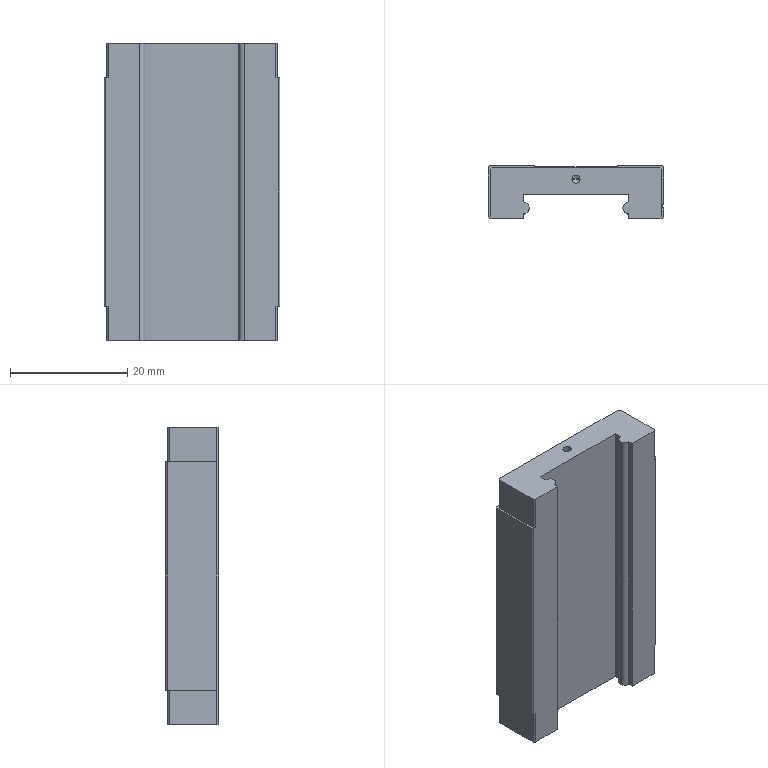Part | NX | features BREP 5 | 1 solid | 94 faces | box 30 x 9.1 x 50.7 mm | volume 9487 mm3 | plane 41 | cylinder 33 | cone 20 | commonest cylinder face diameters 3 x16 2.5 x8 1.4 x4 2 x3 0.6 x2